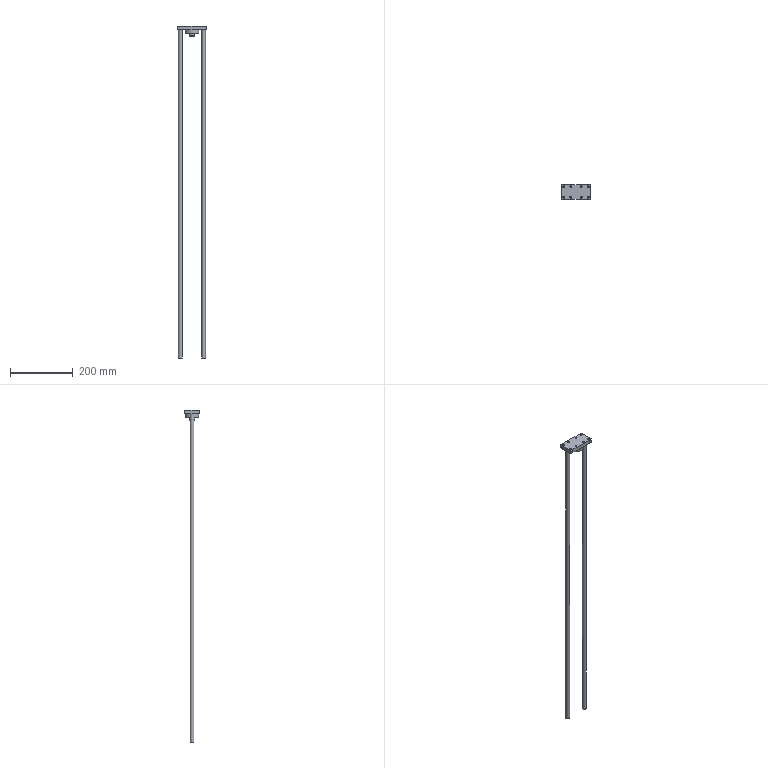Part | STEP file | 150290 FENG-32-400-KF---(JS) | 1 solid | 51 faces | box 90 x 45 x 1055 mm | volume 299074 mm3 | plane 21 | cylinder 18 | cone 12 | commonest cylinder face diameters 4.917 x4 6.6 x4 11 x4 12 x2 17 x2 8.647 x1